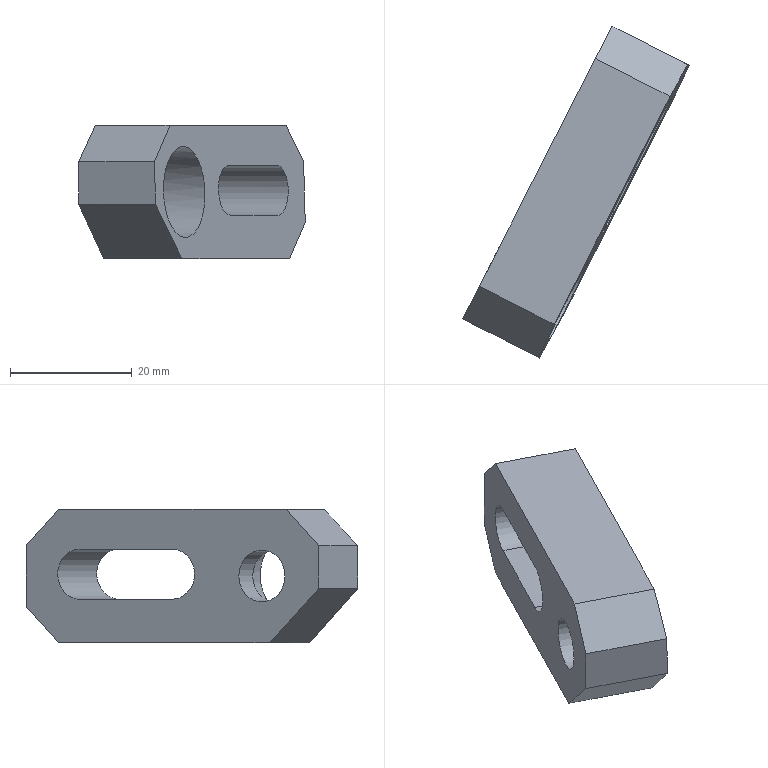Part | STEP file | gslz 2016.10.28-13_id1782_x_t | 1 solid | 17 faces | box 37.214 x 54.544 x 22 mm | volume 10797 mm3 | plane 13 | cylinder 2 | spline 2 | commonest cylinder face diameters 8.5 x1 15 x1